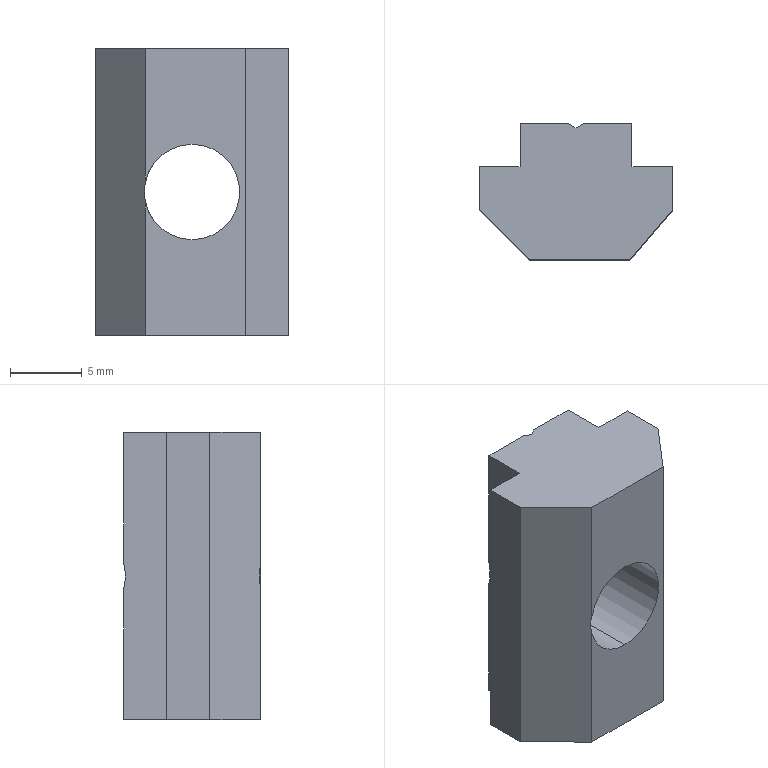Part | SolidWorks | features BaseBody 1 | 1 solid | 23 faces | box 13.5 x 9.5 x 20 mm | volume 1659 mm3 | plane 19 | cylinder 2 | cone 2 | commonest cylinder face diameters 6.647 x2
STEP:
#1=CARTESIAN_POINT('',(0.,0.,-3.324));
#2=VERTEX_POINT('',#1);
#3=CARTESIAN_POINT('',(-3.25,0.,-0.6951));
#4=VERTEX_POINT('',#3);
#5=CARTESIAN_POINT('',(0.,0.,0.));
#6=DIRECTION('',(0.,1.,0.));
#7=DIRECTION('',(0.,0.,1.));
#8=AXIS2_PLACEMENT_3D('',#5,#6,#7);
#9=CIRCLE('',#8,3.324);
#10=EDGE_CURVE('',#2,#4,#9,.T.);
#11=ORIENTED_EDGE('',*,*,#10,.F.);
#12=CARTESIAN_POINT('',(0.,8.823,-3.324));
#13=VERTEX_POINT('',#12);
#14=CARTESIAN_POINT('',(0.,0.,-3.324));
#15=DIRECTION('',(0.,1.,0.));
#16=VECTOR('',#15,1000.);
#17=LINE('',#14,#16);
#18=EDGE_CURVE('',#2,#13,#17,.T.);
#19=ORIENTED_EDGE('',*,*,#18,.T.);
#20=CARTESIAN_POINT('',(0.,8.823,3.324));
#21=VERTEX_POINT('',#20);
#22=CARTESIAN_POINT('',(0.,8.823,0.));
#23=DIRECTION('',(0.,-1.,0.));
#24=DIRECTION('',(0.,0.,1.));
#25=AXIS2_PLACEMENT_3D('',#22,#23,#24);
#26=CIRCLE('',#25,3.324);
#27=EDGE_CURVE('',#21,#13,#26,.T.);
#28=ORIENTED_EDGE('',*,*,#27,.F.);
#29=CARTESIAN_POINT('',(0.,0.,3.324));
#30=VERTEX_POINT('',#29);
#31=CARTESIAN_POINT('',(0.,0.,3.324));
#32=DIRECTION('',(0.,1.,0.));
#33=VECTOR('',#32,1000.);
#34=LINE('',#31,#33);
#35=EDGE_CURVE('',#30,#21,#34,.T.);
#36=ORIENTED_EDGE('',*,*,#35,.F.);
#37=CARTESIAN_POINT('',(-3.25,0.,0.6951));
#38=VERTEX_POINT('',#37);
#39=CARTESIAN_POINT('',(0.,0.,0.));
#40=DIRECTION('',(0.,1.,0.));
#41=DIRECTION('',(0.,0.,1.));
#42=AXIS2_PLACEMENT_3D('',#39,#40,#41);
#43=CIRCLE('',#42,3.324);
#44=EDGE_CURVE('',#38,#30,#43,.T.);
#45=ORIENTED_EDGE('',*,*,#44,.F.);
#46=CARTESIAN_POINT('',(-3.25,0.,0.6951));
#47=CARTESIAN_POINT('',(-3.348,0.09837,0.2352));
#48=CARTESIAN_POINT('',(-3.348,0.09837,-0.2352));
#49=CARTESIAN_POINT('',(-3.25,0.,-0.6951));
#50=(BOUNDED_CURVE()B_SPLINE_CURVE(3,(#46,#47,#48,#49),.UNSPECIFIED.,.F.,.F.)B_SPLINE_CURVE_WITH_KNOTS((4,4),(6.072,6.494),.UNSPECIFIED.)CURVE()GEOMETRIC_REPRESENTATION_ITEM()RATIONAL_B_SPLINE_CURVE((1.,0.9853,0.9853,1.))REPRESENTATION_ITEM(''));
#51=EDGE_CURVE('',#38,#4,#50,.T.);
#52=ORIENTED_EDGE('',*,*,#51,.T.);
#53=EDGE_LOOP('',(#11,#19,#28,#36,#45,#52));
#54=FACE_OUTER_BOUND('',#53,.T.);
#55=CARTESIAN_POINT('',(0.,0.,0.));
#56=DIRECTION('',(0.,1.,0.));
#57=DIRECTION('',(0.,0.,1.));
#58=AXIS2_PLACEMENT_3D('',#55,#56,#57);
#59=CYLINDRICAL_SURFACE('',#58,3.324);
#60=ADVANCED_FACE('',(#54),#59,.F.);
#61=ORIENTED_EDGE('',*,*,#27,.T.);
#62=CARTESIAN_POINT('',(0.,9.2,-3.7));
#63=VERTEX_POINT('',#62);
#64=CARTESIAN_POINT('',(0.,9.5,-4.));
#65=DIRECTION('',(0.,0.7071,-0.7071));
#66=VECTOR('',#65,1000.);
#67=LINE('',#64,#66);
#68=EDGE_CURVE('',#13,#63,#67,.T.);
#69=ORIENTED_EDGE('',*,*,#68,.T.);
#70=CARTESIAN_POINT('',(-0.5,9.5,-3.969));
#71=VERTEX_POINT('',#70);
#72=CARTESIAN_POINT('',(0.,9.2,-3.7));
#73=CARTESIAN_POINT('',(-0.1608,9.296,-3.796));
#74=CARTESIAN_POINT('',(-0.3276,9.397,-3.886));
#75=CARTESIAN_POINT('',(-0.5,9.5,-3.969));
#76=(BOUNDED_CURVE()B_SPLINE_CURVE(3,(#72,#73,#74,#75),.UNSPECIFIED.,.F.,.F.)B_SPLINE_CURVE_WITH_KNOTS((4,4),(4.069,4.173),.UNSPECIFIED.)CURVE()GEOMETRIC_REPRESENTATION_ITEM()RATIONAL_B_SPLINE_CURVE((1.,0.9991,0.9991,1.))REPRESENTATION_ITEM(''));
#77=EDGE_CURVE('',#63,#71,#76,.T.);
#78=ORIENTED_EDGE('',*,*,#77,.T.);
#79=CARTESIAN_POINT('',(-3.9,9.5,-0.8888));
#80=VERTEX_POINT('',#79);
#81=CARTESIAN_POINT('',(0.,9.5,0.));
#82=DIRECTION('',(0.,-1.,0.));
#83=DIRECTION('',(0.,0.,1.));
#84=AXIS2_PLACEMENT_3D('',#81,#82,#83);
#85=CIRCLE('',#84,4.);
#86=EDGE_CURVE('',#80,#71,#85,.T.);
#87=ORIENTED_EDGE('',*,*,#86,.F.);
#88=CARTESIAN_POINT('',(-3.9,9.5,0.8888));
#89=VERTEX_POINT('',#88);
#90=CARTESIAN_POINT('',(-3.9,9.5,0.8888));
#91=CARTESIAN_POINT('',(-3.9,9.435,0.5958));
#92=CARTESIAN_POINT('',(-3.9,9.4,0.3005));
#93=CARTESIAN_POINT('',(-3.9,9.4,-0.2953));
#94=CARTESIAN_POINT('',(-3.9,9.435,-0.5956));
#95=CARTESIAN_POINT('',(-3.9,9.5,-0.8888));
#96=B_SPLINE_CURVE_WITH_KNOTS('',3,(#90,#91,#92,#93,#94,#95),.UNSPECIFIED.,.F.,.F.,(4,2,4),(0.,0.0008912,0.001782),.UNSPECIFIED.);
#97=EDGE_CURVE('',#89,#80,#96,.T.);
#98=ORIENTED_EDGE('',*,*,#97,.F.);
#99=CARTESIAN_POINT('',(-0.5,9.5,3.969));
#100=VERTEX_POINT('',#99);
#101=CARTESIAN_POINT('',(0.,9.5,0.));
#102=DIRECTION('',(0.,-1.,0.));
#103=DIRECTION('',(0.,0.,1.));
#104=AXIS2_PLACEMENT_3D('',#101,#102,#103);
#105=CIRCLE('',#104,4.);
#106=EDGE_CURVE('',#100,#89,#105,.T.);
#107=ORIENTED_EDGE('',*,*,#106,.F.);
#108=CARTESIAN_POINT('',(0.,9.2,3.7));
#109=VERTEX_POINT('',#108);
#110=CARTESIAN_POINT('',(-0.5,9.5,3.969));
#111=CARTESIAN_POINT('',(-0.3276,9.397,3.886));
#112=CARTESIAN_POINT('',(-0.1608,9.296,3.796));
#113=CARTESIAN_POINT('',(0.,9.2,3.7));
#114=(BOUNDED_CURVE()B_SPLINE_CURVE(3,(#110,#111,#112,#113),.UNSPECIFIED.,.F.,.F.)B_SPLINE_CURVE_WITH_KNOTS((4,4),(2.11,2.214),.UNSPECIFIED.)CURVE()GEOMETRIC_REPRESENTATION_ITEM()RATIONAL_B_SPLINE_CURVE((1.,0.9991,0.9991,1.))REPRESENTATION_ITEM(''));
#115=EDGE_CURVE('',#100,#109,#114,.T.);
#116=ORIENTED_EDGE('',*,*,#115,.T.);
#117=CARTESIAN_POINT('',(0.,9.5,4.));
#118=DIRECTION('',(0.,0.7071,0.7071));
#119=VECTOR('',#118,1000.);
#120=LINE('',#117,#119);
#121=EDGE_CURVE('',#21,#109,#120,.T.);
#122=ORIENTED_EDGE('',*,*,#121,.F.);
#123=EDGE_LOOP('',(#61,#69,#78,#87,#98,#107,#116,#122));
#124=FACE_OUTER_BOUND('',#123,.T.);
#125=CARTESIAN_POINT('',(0.,9.5,0.));
#126=DIRECTION('',(0.,1.,0.));
#127=DIRECTION('',(0.,0.,1.));
#128=AXIS2_PLACEMENT_3D('',#125,#126,#127);
#129=CONICAL_SURFACE('',#128,4.,0.7854);
#130=ADVANCED_FACE('',(#124),#129,.F.);
#131=ORIENTED_EDGE('',*,*,#18,.F.);
#132=CARTESIAN_POINT('',(0.,0.,0.));
#133=DIRECTION('',(0.,1.,0.));
#134=DIRECTION('',(0.,0.,1.));
#135=AXIS2_PLACEMENT_3D('',#132,#133,#134);
#136=CIRCLE('',#135,3.324);
#137=EDGE_CURVE('',#30,#2,#136,.T.);
#138=ORIENTED_EDGE('',*,*,#137,.F.);
#139=ORIENTED_EDGE('',*,*,#35,.T.);
#140=CARTESIAN_POINT('',(0.,8.823,0.));
#141=DIRECTION('',(0.,-1.,0.));
#142=DIRECTION('',(0.,0.,1.));
#143=AXIS2_PLACEMENT_3D('',#140,#141,#142);
#144=CIRCLE('',#143,3.324);
#145=EDGE_CURVE('',#13,#21,#144,.T.);
#146=ORIENTED_EDGE('',*,*,#145,.F.);
#147=EDGE_LOOP('',(#131,#138,#139,#146));
#148=FACE_OUTER_BOUND('',#147,.T.);
#149=CARTESIAN_POINT('',(0.,0.,0.));
#150=DIRECTION('',(0.,1.,0.));
#151=DIRECTION('',(0.,0.,1.));
#152=AXIS2_PLACEMENT_3D('',#149,#150,#151);
#153=CYLINDRICAL_SURFACE('',#152,3.324);
#154=ADVANCED_FACE('',(#148),#153,.F.);
#155=ORIENTED_EDGE('',*,*,#68,.F.);
#156=ORIENTED_EDGE('',*,*,#145,.T.);
#157=ORIENTED_EDGE('',*,*,#121,.T.);
#158=CARTESIAN_POINT('',(0.5,9.5,3.969));
#159=VERTEX_POINT('',#158);
#160=CARTESIAN_POINT('',(0.,9.2,3.7));
#161=CARTESIAN_POINT('',(0.1608,9.296,3.796));
#162=CARTESIAN_POINT('',(0.3276,9.397,3.886));
#163=CARTESIAN_POINT('',(0.5,9.5,3.969));
#164=(BOUNDED_CURVE()B_SPLINE_CURVE(3,(#160,#161,#162,#163),.UNSPECIFIED.,.F.,.F.)B_SPLINE_CURVE_WITH_KNOTS((4,4),(4.069,4.173),.UNSPECIFIED.)CURVE()GEOMETRIC_REPRESENTATION_ITEM()RATIONAL_B_SPLINE_CURVE((1.,0.9991,0.9991,1.))REPRESENTATION_ITEM(''));
#165=EDGE_CURVE('',#109,#159,#164,.T.);
#166=ORIENTED_EDGE('',*,*,#165,.T.);
#167=CARTESIAN_POINT('',(3.9,9.5,0.8888));
#168=VERTEX_POINT('',#167);
#169=CARTESIAN_POINT('',(0.,9.5,0.));
#170=DIRECTION('',(0.,-1.,0.));
#171=DIRECTION('',(0.,0.,1.));
#172=AXIS2_PLACEMENT_3D('',#169,#170,#171);
#173=CIRCLE('',#172,4.);
#174=EDGE_CURVE('',#168,#159,#173,.T.);
#175=ORIENTED_EDGE('',*,*,#174,.F.);
#176=CARTESIAN_POINT('',(3.9,9.5,-0.8888));
#177=VERTEX_POINT('',#176);
#178=CARTESIAN_POINT('',(3.9,9.5,-0.8888));
#179=CARTESIAN_POINT('',(3.9,9.435,-0.5958));
#180=CARTESIAN_POINT('',(3.9,9.4,-0.3005));
#181=CARTESIAN_POINT('',(3.9,9.4,0.2953));
#182=CARTESIAN_POINT('',(3.9,9.435,0.5956));
#183=CARTESIAN_POINT('',(3.9,9.5,0.8888));
#184=B_SPLINE_CURVE_WITH_KNOTS('',3,(#178,#179,#180,#181,#182,#183),.UNSPECIFIED.,.F.,.F.,(4,2,4),(0.,0.0008912,0.001782),.UNSPECIFIED.);
#185=EDGE_CURVE('',#177,#168,#184,.T.);
#186=ORIENTED_EDGE('',*,*,#185,.F.);
#187=CARTESIAN_POINT('',(0.5,9.5,-3.969));
#188=VERTEX_POINT('',#187);
#189=CARTESIAN_POINT('',(0.,9.5,0.));
#190=DIRECTION('',(0.,-1.,0.));
#191=DIRECTION('',(0.,0.,1.));
#192=AXIS2_PLACEMENT_3D('',#189,#190,#191);
#193=CIRCLE('',#192,4.);
#194=EDGE_CURVE('',#188,#177,#193,.T.);
#195=ORIENTED_EDGE('',*,*,#194,.F.);
#196=CARTESIAN_POINT('',(0.5,9.5,-3.969));
#197=CARTESIAN_POINT('',(0.3276,9.397,-3.886));
#198=CARTESIAN_POINT('',(0.1608,9.296,-3.796));
#199=CARTESIAN_POINT('',(0.,9.2,-3.7));
#200=(BOUNDED_CURVE()B_SPLINE_CURVE(3,(#196,#197,#198,#199),.UNSPECIFIED.,.F.,.F.)B_SPLINE_CURVE_WITH_KNOTS((4,4),(2.11,2.214),.UNSPECIFIED.)CURVE()GEOMETRIC_REPRESENTATION_ITEM()RATIONAL_B_SPLINE_CURVE((1.,0.9991,0.9991,1.))REPRESENTATION_ITEM(''));
#201=EDGE_CURVE('',#188,#63,#200,.T.);
#202=ORIENTED_EDGE('',*,*,#201,.T.);
#203=EDGE_LOOP('',(#155,#156,#157,#166,#175,#186,#195,#202));
#204=FACE_OUTER_BOUND('',#203,.T.);
#205=CARTESIAN_POINT('',(0.,9.5,0.));
#206=DIRECTION('',(0.,1.,0.));
#207=DIRECTION('',(0.,0.,1.));
#208=AXIS2_PLACEMENT_3D('',#205,#206,#207);
#209=CONICAL_SURFACE('',#208,4.,0.7854);
#210=ADVANCED_FACE('',(#204),#209,.F.);
#211=ORIENTED_EDGE('',*,*,#44,.T.);
#212=ORIENTED_EDGE('',*,*,#137,.T.);
#213=ORIENTED_EDGE('',*,*,#10,.T.);
#214=CARTESIAN_POINT('',(-3.25,0.,-10.));
#215=VERTEX_POINT('',#214);
#216=CARTESIAN_POINT('',(-3.25,0.,10.));
#217=DIRECTION('',(0.,0.,1.));
#218=VECTOR('',#217,1000.);
#219=LINE('',#216,#218);
#220=EDGE_CURVE('',#215,#4,#219,.T.);
#221=ORIENTED_EDGE('',*,*,#220,.F.);
#222=CARTESIAN_POINT('',(3.75,0.,-10.));
#223=VERTEX_POINT('',#222);
#224=CARTESIAN_POINT('',(-3.25,0.,-10.));
#225=DIRECTION('',(-1.,0.,0.));
#226=VECTOR('',#225,1000.);
#227=LINE('',#224,#226);
#228=EDGE_CURVE('',#223,#215,#227,.T.);
#229=ORIENTED_EDGE('',*,*,#228,.F.);
#230=CARTESIAN_POINT('',(3.75,0.,10.));
#231=VERTEX_POINT('',#230);
#232=CARTESIAN_POINT('',(3.75,0.,10.));
#233=DIRECTION('',(0.,0.,-1.));
#234=VECTOR('',#233,1000.);
#235=LINE('',#232,#234);
#236=EDGE_CURVE('',#231,#223,#235,.T.);
#237=ORIENTED_EDGE('',*,*,#236,.F.);
#238=CARTESIAN_POINT('',(-3.25,0.,10.));
#239=VERTEX_POINT('',#238);
#240=CARTESIAN_POINT('',(-3.25,0.,10.));
#241=DIRECTION('',(1.,0.,0.));
#242=VECTOR('',#241,1000.);
#243=LINE('',#240,#242);
#244=EDGE_CURVE('',#239,#231,#243,.T.);
#245=ORIENTED_EDGE('',*,*,#244,.F.);
#246=CARTESIAN_POINT('',(-3.25,0.,10.));
#247=DIRECTION('',(0.,0.,1.));
#248=VECTOR('',#247,1000.);
#249=LINE('',#246,#248);
#250=EDGE_CURVE('',#38,#239,#249,.T.);
#251=ORIENTED_EDGE('',*,*,#250,.F.);
#252=EDGE_LOOP('',(#211,#212,#213,#221,#229,#237,#245,#251));
#253=FACE_OUTER_BOUND('',#252,.T.);
#254=CARTESIAN_POINT('',(-3.25,0.,10.));
#255=DIRECTION('',(0.,1.,0.));
#256=DIRECTION('',(0.,0.,1.));
#257=AXIS2_PLACEMENT_3D('',#254,#255,#256);
#258=PLANE('',#257);
#259=ADVANCED_FACE('',(#253),#258,.F.);
#260=CARTESIAN_POINT('',(3.9,9.5,10.));
#261=VERTEX_POINT('',#260);
#262=CARTESIAN_POINT('',(3.9,9.5,10.));
#263=DIRECTION('',(0.,0.,-1.));
#264=VECTOR('',#263,1000.);
#265=LINE('',#262,#264);
#266=EDGE_CURVE('',#261,#168,#265,.T.);
#267=ORIENTED_EDGE('',*,*,#266,.F.);
#268=CARTESIAN_POINT('',(3.9,6.5,10.));
#269=VERTEX_POINT('',#268);
#270=CARTESIAN_POINT('',(3.9,6.5,10.));
#271=DIRECTION('',(0.,1.,0.));
#272=VECTOR('',#271,1000.);
#273=LINE('',#270,#272);
#274=EDGE_CURVE('',#269,#261,#273,.T.);
#275=ORIENTED_EDGE('',*,*,#274,.F.);
#276=CARTESIAN_POINT('',(3.9,6.5,-10.));
#277=VERTEX_POINT('',#276);
#278=CARTESIAN_POINT('',(3.9,6.5,10.));
#279=DIRECTION('',(0.,0.,1.));
#280=VECTOR('',#279,1000.);
#281=LINE('',#278,#280);
#282=EDGE_CURVE('',#277,#269,#281,.T.);
#283=ORIENTED_EDGE('',*,*,#282,.F.);
#284=CARTESIAN_POINT('',(3.9,9.5,-10.));
#285=VERTEX_POINT('',#284);
#286=CARTESIAN_POINT('',(3.9,6.5,-10.));
#287=DIRECTION('',(0.,-1.,0.));
#288=VECTOR('',#287,1000.);
#289=LINE('',#286,#288);
#290=EDGE_CURVE('',#285,#277,#289,.T.);
#291=ORIENTED_EDGE('',*,*,#290,.F.);
#292=CARTESIAN_POINT('',(3.9,9.5,10.));
#293=DIRECTION('',(0.,0.,-1.));
#294=VECTOR('',#293,1000.);
#295=LINE('',#292,#294);
#296=EDGE_CURVE('',#177,#285,#295,.T.);
#297=ORIENTED_EDGE('',*,*,#296,.F.);
#298=ORIENTED_EDGE('',*,*,#185,.T.);
#299=EDGE_LOOP('',(#267,#275,#283,#291,#297,#298));
#300=FACE_OUTER_BOUND('',#299,.T.);
#301=CARTESIAN_POINT('',(3.9,6.5,10.));
#302=DIRECTION('',(-1.,0.,0.));
#303=DIRECTION('',(0.,-1.,0.));
#304=AXIS2_PLACEMENT_3D('',#301,#302,#303);
#305=PLANE('',#304);
#306=ADVANCED_FACE('',(#300),#305,.F.);
#307=ORIENTED_EDGE('',*,*,#296,.T.);
#308=CARTESIAN_POINT('',(0.5,9.5,-10.));
#309=VERTEX_POINT('',#308);
#310=CARTESIAN_POINT('',(3.9,9.5,-10.));
#311=DIRECTION('',(1.,0.,0.));
#312=VECTOR('',#311,1000.);
#313=LINE('',#310,#312);
#314=EDGE_CURVE('',#309,#285,#313,.T.);
#315=ORIENTED_EDGE('',*,*,#314,.F.);
#316=CARTESIAN_POINT('',(0.5,9.5,10.));
#317=DIRECTION('',(0.,0.,-1.));
#318=VECTOR('',#317,1000.);
#319=LINE('',#316,#318);
#320=EDGE_CURVE('',#188,#309,#319,.T.);
#321=ORIENTED_EDGE('',*,*,#320,.F.);
#322=ORIENTED_EDGE('',*,*,#194,.T.);
#323=EDGE_LOOP('',(#307,#315,#321,#322));
#324=FACE_OUTER_BOUND('',#323,.T.);
#325=CARTESIAN_POINT('',(3.9,9.5,10.));
#326=DIRECTION('',(0.,-1.,0.));
#327=DIRECTION('',(0.,0.,-1.));
#328=AXIS2_PLACEMENT_3D('',#325,#326,#327);
#329=PLANE('',#328);
#330=ADVANCED_FACE('',(#324),#329,.F.);
#331=CARTESIAN_POINT('',(-0.5,9.5,-10.));
#332=VERTEX_POINT('',#331);
#333=CARTESIAN_POINT('',(-0.5,9.5,10.));
#334=DIRECTION('',(0.,0.,1.));
#335=VECTOR('',#334,1000.);
#336=LINE('',#333,#335);
#337=EDGE_CURVE('',#332,#71,#336,.T.);
#338=ORIENTED_EDGE('',*,*,#337,.F.);
#339=CARTESIAN_POINT('',(-3.9,9.5,-10.));
#340=VERTEX_POINT('',#339);
#341=CARTESIAN_POINT('',(-0.5,9.5,-10.));
#342=DIRECTION('',(1.,0.,0.));
#343=VECTOR('',#342,1000.);
#344=LINE('',#341,#343);
#345=EDGE_CURVE('',#340,#332,#344,.T.);
#346=ORIENTED_EDGE('',*,*,#345,.F.);
#347=CARTESIAN_POINT('',(-3.9,9.5,10.));
#348=DIRECTION('',(0.,0.,-1.));
#349=VECTOR('',#348,1000.);
#350=LINE('',#347,#349);
#351=EDGE_CURVE('',#80,#340,#350,.T.);
#352=ORIENTED_EDGE('',*,*,#351,.F.);
#353=ORIENTED_EDGE('',*,*,#86,.T.);
#354=EDGE_LOOP('',(#338,#346,#352,#353));
#355=FACE_OUTER_BOUND('',#354,.T.);
#356=CARTESIAN_POINT('',(-0.5,9.5,10.));
#357=DIRECTION('',(0.,-1.,0.));
#358=DIRECTION('',(0.,0.,-1.));
#359=AXIS2_PLACEMENT_3D('',#356,#357,#358);
#360=PLANE('',#359);
#361=ADVANCED_FACE('',(#355),#360,.F.);
#362=ORIENTED_EDGE('',*,*,#351,.T.);
#363=CARTESIAN_POINT('',(-3.9,6.5,-10.));
#364=VERTEX_POINT('',#363);
#365=CARTESIAN_POINT('',(-3.9,9.5,-10.));
#366=DIRECTION('',(0.,1.,0.));
#367=VECTOR('',#366,1000.);
#368=LINE('',#365,#367);
#369=EDGE_CURVE('',#364,#340,#368,.T.);
#370=ORIENTED_EDGE('',*,*,#369,.F.);
#371=CARTESIAN_POINT('',(-3.9,6.5,10.));
#372=VERTEX_POINT('',#371);
#373=CARTESIAN_POINT('',(-3.9,6.5,10.));
#374=DIRECTION('',(0.,0.,-1.));
#375=VECTOR('',#374,1000.);
#376=LINE('',#373,#375);
#377=EDGE_CURVE('',#372,#364,#376,.T.);
#378=ORIENTED_EDGE('',*,*,#377,.F.);
#379=CARTESIAN_POINT('',(-3.9,9.5,10.));
#380=VERTEX_POINT('',#379);
#381=CARTESIAN_POINT('',(-3.9,9.5,10.));
#382=DIRECTION('',(0.,-1.,0.));
#383=VECTOR('',#382,1000.);
#384=LINE('',#381,#383);
#385=EDGE_CURVE('',#380,#372,#384,.T.);
#386=ORIENTED_EDGE('',*,*,#385,.F.);
#387=CARTESIAN_POINT('',(-3.9,9.5,10.));
#388=DIRECTION('',(0.,0.,1.));
#389=VECTOR('',#388,1000.);
#390=LINE('',#387,#389);
#391=EDGE_CURVE('',#89,#380,#390,.T.);
#392=ORIENTED_EDGE('',*,*,#391,.F.);
#393=ORIENTED_EDGE('',*,*,#97,.T.);
#394=EDGE_LOOP('',(#362,#370,#378,#386,#392,#393));
#395=FACE_OUTER_BOUND('',#394,.T.);
#396=CARTESIAN_POINT('',(-3.9,9.5,10.));
#397=DIRECTION('',(1.,0.,0.));
#398=DIRECTION('',(0.,1.,0.));
#399=AXIS2_PLACEMENT_3D('',#396,#397,#398);
#400=PLANE('',#399);
#401=ADVANCED_FACE('',(#395),#400,.F.);
#402=ORIENTED_EDGE('',*,*,#391,.T.);
#403=CARTESIAN_POINT('',(-0.5,9.5,10.));
#404=VERTEX_POINT('',#403);
#405=CARTESIAN_POINT('',(-0.5,9.5,10.));
#406=DIRECTION('',(-1.,0.,0.));
#407=VECTOR('',#406,1000.);
#408=LINE('',#405,#407);
#409=EDGE_CURVE('',#404,#380,#408,.T.);
#410=ORIENTED_EDGE('',*,*,#409,.F.);
#411=CARTESIAN_POINT('',(-0.5,9.5,10.));
#412=DIRECTION('',(0.,0.,1.));
#413=VECTOR('',#412,1000.);
#414=LINE('',#411,#413);
#415=EDGE_CURVE('',#100,#404,#414,.T.);
#416=ORIENTED_EDGE('',*,*,#415,.F.);
#417=ORIENTED_EDGE('',*,*,#106,.T.);
#418=EDGE_LOOP('',(#402,#410,#416,#417));
#419=FACE_OUTER_BOUND('',#418,.T.);
#420=CARTESIAN_POINT('',(-0.5,9.5,10.));
#421=DIRECTION('',(0.,-1.,0.));
#422=DIRECTION('',(0.,0.,-1.));
#423=AXIS2_PLACEMENT_3D('',#420,#421,#422);
#424=PLANE('',#423);
#425=ADVANCED_FACE('',(#419),#424,.F.);
#426=CARTESIAN_POINT('',(0.5,9.5,10.));
#427=VERTEX_POINT('',#426);
#428=CARTESIAN_POINT('',(0.5,9.5,10.));
#429=DIRECTION('',(0.,0.,-1.));
#430=VECTOR('',#429,1000.);
#431=LINE('',#428,#430);
#432=EDGE_CURVE('',#427,#159,#431,.T.);
#433=ORIENTED_EDGE('',*,*,#432,.F.);
#434=CARTESIAN_POINT('',(3.9,9.5,10.));
#435=DIRECTION('',(-1.,0.,0.));
#436=VECTOR('',#435,1000.);
#437=LINE('',#434,#436);
#438=EDGE_CURVE('',#261,#427,#437,.T.);
#439=ORIENTED_EDGE('',*,*,#438,.F.);
#440=ORIENTED_EDGE('',*,*,#266,.T.);
#441=ORIENTED_EDGE('',*,*,#174,.T.);
#442=EDGE_LOOP('',(#433,#439,#440,#441));
#443=FACE_OUTER_BOUND('',#442,.T.);
#444=CARTESIAN_POINT('',(3.9,9.5,10.));
#445=DIRECTION('',(0.,-1.,0.));
#446=DIRECTION('',(0.,0.,-1.));
#447=AXIS2_PLACEMENT_3D('',#444,#445,#446);
#448=PLANE('',#447);
#449=ADVANCED_FACE('',(#443),#448,.F.);
#450=ORIENTED_EDGE('',*,*,#250,.T.);
#451=CARTESIAN_POINT('',(-6.75,3.5,10.));
#452=VERTEX_POINT('',#451);
#453=CARTESIAN_POINT('',(-6.75,3.5,10.));
#454=DIRECTION('',(0.7071,-0.7071,0.));
#455=VECTOR('',#454,1000.);
#456=LINE('',#453,#455);
#457=EDGE_CURVE('',#452,#239,#456,.T.);
#458=ORIENTED_EDGE('',*,*,#457,.F.);
#459=CARTESIAN_POINT('',(-6.75,3.5,-10.));
#460=VERTEX_POINT('',#459);
#461=CARTESIAN_POINT('',(-6.75,3.5,10.));
#462=DIRECTION('',(0.,0.,1.));
#463=VECTOR('',#462,1000.);
#464=LINE('',#461,#463);
#465=EDGE_CURVE('',#460,#452,#464,.T.);
#466=ORIENTED_EDGE('',*,*,#465,.F.);
#467=CARTESIAN_POINT('',(-6.75,3.5,-10.));
#468=DIRECTION('',(-0.7071,0.7071,0.));
#469=VECTOR('',#468,1000.);
#470=LINE('',#467,#469);
#471=EDGE_CURVE('',#215,#460,#470,.T.);
#472=ORIENTED_EDGE('',*,*,#471,.F.);
#473=ORIENTED_EDGE('',*,*,#220,.T.);
#474=ORIENTED_EDGE('',*,*,#51,.F.);
#475=EDGE_LOOP('',(#450,#458,#466,#472,#473,#474));
#476=FACE_OUTER_BOUND('',#475,.T.);
#477=CARTESIAN_POINT('',(-6.75,3.5,10.));
#478=DIRECTION('',(0.7071,0.7071,0.));
#479=DIRECTION('',(-0.7071,0.7071,0.));
#480=AXIS2_PLACEMENT_3D('',#477,#478,#479);
#481=PLANE('',#480);
#482=ADVANCED_FACE('',(#476),#481,.F.);
#483=CARTESIAN_POINT('',(-6.75,6.5,-10.));
#484=VERTEX_POINT('',#483);
#485=CARTESIAN_POINT('',(0.,6.5,-10.));
#486=DIRECTION('',(-1.,0.,0.));
#487=VECTOR('',#486,1000.);
#488=LINE('',#485,#487);
#489=EDGE_CURVE('',#364,#484,#488,.T.);
#490=ORIENTED_EDGE('',*,*,#489,.F.);
#491=ORIENTED_EDGE('',*,*,#369,.T.);
#492=ORIENTED_EDGE('',*,*,#345,.T.);
#493=CARTESIAN_POINT('',(0.,9.2,-10.));
#494=VERTEX_POINT('',#493);
#495=CARTESIAN_POINT('',(0.,9.2,-10.));
#496=DIRECTION('',(-0.8575,0.5145,0.));
#497=VECTOR('',#496,1000.);
#498=LINE('',#495,#497);
#499=EDGE_CURVE('',#494,#332,#498,.T.);
#500=ORIENTED_EDGE('',*,*,#499,.F.);
#501=CARTESIAN_POINT('',(0.5,9.5,-10.));
#502=DIRECTION('',(-0.8575,-0.5145,0.));
#503=VECTOR('',#502,1000.);
#504=LINE('',#501,#503);
#505=EDGE_CURVE('',#309,#494,#504,.T.);
#506=ORIENTED_EDGE('',*,*,#505,.F.);
#507=ORIENTED_EDGE('',*,*,#314,.T.);
#508=ORIENTED_EDGE('',*,*,#290,.T.);
#509=CARTESIAN_POINT('',(6.75,6.5,-10.));
#510=VERTEX_POINT('',#509);
#511=CARTESIAN_POINT('',(0.,6.5,-10.));
#512=DIRECTION('',(-1.,0.,0.));
#513=VECTOR('',#512,1000.);
#514=LINE('',#511,#513);
#515=EDGE_CURVE('',#510,#277,#514,.T.);
#516=ORIENTED_EDGE('',*,*,#515,.F.);
#517=CARTESIAN_POINT('',(6.75,3.5,-10.));
#518=VERTEX_POINT('',#517);
#519=CARTESIAN_POINT('',(6.75,0.,-10.));
#520=DIRECTION('',(0.,1.,0.));
#521=VECTOR('',#520,1000.);
#522=LINE('',#519,#521);
#523=EDGE_CURVE('',#518,#510,#522,.T.);
#524=ORIENTED_EDGE('',*,*,#523,.F.);
#525=CARTESIAN_POINT('',(3.75,0.,-10.));
#526=DIRECTION('',(0.6508,0.7593,0.));
#527=VECTOR('',#526,1000.);
#528=LINE('',#525,#527);
#529=EDGE_CURVE('',#223,#518,#528,.T.);
#530=ORIENTED_EDGE('',*,*,#529,.F.);
#531=ORIENTED_EDGE('',*,*,#228,.T.);
#532=ORIENTED_EDGE('',*,*,#471,.T.);
#533=CARTESIAN_POINT('',(-6.75,0.,-10.));
#534=DIRECTION('',(0.,-1.,0.));
#535=VECTOR('',#534,1000.);
#536=LINE('',#533,#535);
#537=EDGE_CURVE('',#484,#460,#536,.T.);
#538=ORIENTED_EDGE('',*,*,#537,.F.);
#539=EDGE_LOOP('',(#490,#491,#492,#500,#506,#507,#508,#516,#524,#530,#531,#532,#538));
#540=FACE_OUTER_BOUND('',#539,.T.);
#541=CARTESIAN_POINT('',(0.,0.,-10.));
#542=DIRECTION('',(0.,0.,1.));
#543=DIRECTION('',(1.,0.,0.));
#544=AXIS2_PLACEMENT_3D('',#541,#542,#543);
#545=PLANE('',#544);
#546=ADVANCED_FACE('',(#540),#545,.F.);
#547=CARTESIAN_POINT('',(6.75,3.5,10.));
#548=VERTEX_POINT('',#547);
#549=CARTESIAN_POINT('',(6.75,3.5,10.));
#550=DIRECTION('',(0.,0.,-1.));
#551=VECTOR('',#550,1000.);
#552=LINE('',#549,#551);
#553=EDGE_CURVE('',#548,#518,#552,.T.);
#554=ORIENTED_EDGE('',*,*,#553,.F.);
#555=CARTESIAN_POINT('',(3.75,0.,10.));
#556=DIRECTION('',(0.6508,0.7593,0.));
#557=VECTOR('',#556,1000.);
#558=LINE('',#555,#557);
#559=EDGE_CURVE('',#231,#548,#558,.T.);
#560=ORIENTED_EDGE('',*,*,#559,.F.);
#561=ORIENTED_EDGE('',*,*,#236,.T.);
#562=ORIENTED_EDGE('',*,*,#529,.T.);
#563=EDGE_LOOP('',(#554,#560,#561,#562));
#564=FACE_OUTER_BOUND('',#563,.T.);
#565=CARTESIAN_POINT('',(3.75,0.,10.));
#566=DIRECTION('',(-0.7593,0.6508,0.));
#567=DIRECTION('',(-0.6508,-0.7593,0.));
#568=AXIS2_PLACEMENT_3D('',#565,#566,#567);
#569=PLANE('',#568);
#570=ADVANCED_FACE('',(#564),#569,.F.);
#571=ORIENTED_EDGE('',*,*,#385,.T.);
#572=CARTESIAN_POINT('',(-6.75,6.5,10.));
#573=VERTEX_POINT('',#572);
#574=CARTESIAN_POINT('',(0.,6.5,10.));
#575=DIRECTION('',(-1.,0.,0.));
#576=VECTOR('',#575,1000.);
#577=LINE('',#574,#576);
#578=EDGE_CURVE('',#372,#573,#577,.T.);
#579=ORIENTED_EDGE('',*,*,#578,.T.);
#580=CARTESIAN_POINT('',(-6.75,0.,10.));
#581=DIRECTION('',(0.,-1.,0.));
#582=VECTOR('',#581,1000.);
#583=LINE('',#580,#582);
#584=EDGE_CURVE('',#573,#452,#583,.T.);
#585=ORIENTED_EDGE('',*,*,#584,.T.);
#586=ORIENTED_EDGE('',*,*,#457,.T.);
#587=ORIENTED_EDGE('',*,*,#244,.T.);
#588=ORIENTED_EDGE('',*,*,#559,.T.);
#589=CARTESIAN_POINT('',(6.75,6.5,10.));
#590=VERTEX_POINT('',#589);
#591=CARTESIAN_POINT('',(6.75,0.,10.));
#592=DIRECTION('',(0.,1.,0.));
#593=VECTOR('',#592,1000.);
#594=LINE('',#591,#593);
#595=EDGE_CURVE('',#548,#590,#594,.T.);
#596=ORIENTED_EDGE('',*,*,#595,.T.);
#597=CARTESIAN_POINT('',(0.,6.5,10.));
#598=DIRECTION('',(-1.,0.,0.));
#599=VECTOR('',#598,1000.);
#600=LINE('',#597,#599);
#601=EDGE_CURVE('',#590,#269,#600,.T.);
#602=ORIENTED_EDGE('',*,*,#601,.T.);
#603=ORIENTED_EDGE('',*,*,#274,.T.);
#604=ORIENTED_EDGE('',*,*,#438,.T.);
#605=CARTESIAN_POINT('',(0.,9.2,10.));
#606=VERTEX_POINT('',#605);
#607=CARTESIAN_POINT('',(0.5,9.5,10.));
#608=DIRECTION('',(-0.8575,-0.5145,0.));
#609=VECTOR('',#608,1000.);
#610=LINE('',#607,#609);
#611=EDGE_CURVE('',#427,#606,#610,.T.);
#612=ORIENTED_EDGE('',*,*,#611,.T.);
#613=CARTESIAN_POINT('',(0.,9.2,10.));
#614=DIRECTION('',(-0.8575,0.5145,0.));
#615=VECTOR('',#614,1000.);
#616=LINE('',#613,#615);
#617=EDGE_CURVE('',#606,#404,#616,.T.);
#618=ORIENTED_EDGE('',*,*,#617,.T.);
#619=ORIENTED_EDGE('',*,*,#409,.T.);
#620=EDGE_LOOP('',(#571,#579,#585,#586,#587,#588,#596,#602,#603,#604,#612,#618,#619));
#621=FACE_OUTER_BOUND('',#620,.T.);
#622=CARTESIAN_POINT('',(0.,0.,10.));
#623=DIRECTION('',(0.,0.,1.));
#624=DIRECTION('',(1.,0.,0.));
#625=AXIS2_PLACEMENT_3D('',#622,#623,#624);
#626=PLANE('',#625);
#627=ADVANCED_FACE('',(#621),#626,.T.);
#628=ORIENTED_EDGE('',*,*,#282,.T.);
#629=ORIENTED_EDGE('',*,*,#601,.F.);
#630=CARTESIAN_POINT('',(6.75,6.5,10.));
#631=DIRECTION('',(0.,0.,1.));
#632=VECTOR('',#631,1000.);
#633=LINE('',#630,#632);
#634=EDGE_CURVE('',#510,#590,#633,.T.);
#635=ORIENTED_EDGE('',*,*,#634,.F.);
#636=ORIENTED_EDGE('',*,*,#515,.T.);
#637=EDGE_LOOP('',(#628,#629,#635,#636));
#638=FACE_OUTER_BOUND('',#637,.T.);
#639=CARTESIAN_POINT('',(6.75,6.5,10.));
#640=DIRECTION('',(0.,-1.,0.));
#641=DIRECTION('',(0.,0.,-1.));
#642=AXIS2_PLACEMENT_3D('',#639,#640,#641);
#643=PLANE('',#642);
#644=ADVANCED_FACE('',(#638),#643,.F.);
#645=ORIENTED_EDGE('',*,*,#320,.T.);
#646=ORIENTED_EDGE('',*,*,#505,.T.);
#647=CARTESIAN_POINT('',(0.,9.2,10.));
#648=DIRECTION('',(0.,0.,-1.));
#649=VECTOR('',#648,1000.);
#650=LINE('',#647,#649);
#651=EDGE_CURVE('',#63,#494,#650,.T.);
#652=ORIENTED_EDGE('',*,*,#651,.F.);
#653=ORIENTED_EDGE('',*,*,#201,.F.);
#654=EDGE_LOOP('',(#645,#646,#652,#653));
#655=FACE_OUTER_BOUND('',#654,.T.);
#656=CARTESIAN_POINT('',(0.5,9.5,10.));
#657=DIRECTION('',(0.5145,-0.8575,0.));
#658=DIRECTION('',(0.8575,0.5145,0.));
#659=AXIS2_PLACEMENT_3D('',#656,#657,#658);
#660=PLANE('',#659);
#661=ADVANCED_FACE('',(#655),#660,.F.);
#662=ORIENTED_EDGE('',*,*,#651,.T.);
#663=ORIENTED_EDGE('',*,*,#499,.T.);
#664=ORIENTED_EDGE('',*,*,#337,.T.);
#665=ORIENTED_EDGE('',*,*,#77,.F.);
#666=EDGE_LOOP('',(#662,#663,#664,#665));
#667=FACE_OUTER_BOUND('',#666,.T.);
#668=CARTESIAN_POINT('',(0.,9.2,10.));
#669=DIRECTION('',(-0.5145,-0.8575,0.));
#670=DIRECTION('',(0.8575,-0.5145,0.));
#671=AXIS2_PLACEMENT_3D('',#668,#669,#670);
#672=PLANE('',#671);
#673=ADVANCED_FACE('',(#667),#672,.F.);
#674=CARTESIAN_POINT('',(-6.75,6.5,10.));
#675=DIRECTION('',(0.,0.,-1.));
#676=VECTOR('',#675,1000.);
#677=LINE('',#674,#676);
#678=EDGE_CURVE('',#573,#484,#677,.T.);
#679=ORIENTED_EDGE('',*,*,#678,.F.);
#680=ORIENTED_EDGE('',*,*,#578,.F.);
#681=ORIENTED_EDGE('',*,*,#377,.T.);
#682=ORIENTED_EDGE('',*,*,#489,.T.);
#683=EDGE_LOOP('',(#679,#680,#681,#682));
#684=FACE_OUTER_BOUND('',#683,.T.);
#685=CARTESIAN_POINT('',(-3.9,6.5,10.));
#686=DIRECTION('',(0.,-1.,0.));
#687=DIRECTION('',(0.,0.,-1.));
#688=AXIS2_PLACEMENT_3D('',#685,#686,#687);
#689=PLANE('',#688);
#690=ADVANCED_FACE('',(#684),#689,.F.);
#691=ORIENTED_EDGE('',*,*,#415,.T.);
#692=ORIENTED_EDGE('',*,*,#617,.F.);
#693=CARTESIAN_POINT('',(0.,9.2,10.));
#694=DIRECTION('',(0.,0.,1.));
#695=VECTOR('',#694,1000.);
#696=LINE('',#693,#695);
#697=EDGE_CURVE('',#109,#606,#696,.T.);
#698=ORIENTED_EDGE('',*,*,#697,.F.);
#699=ORIENTED_EDGE('',*,*,#115,.F.);
#700=EDGE_LOOP('',(#691,#692,#698,#699));
#701=FACE_OUTER_BOUND('',#700,.T.);
#702=CARTESIAN_POINT('',(0.,9.2,10.));
#703=DIRECTION('',(-0.5145,-0.8575,0.));
#704=DIRECTION('',(0.8575,-0.5145,0.));
#705=AXIS2_PLACEMENT_3D('',#702,#703,#704);
#706=PLANE('',#705);
#707=ADVANCED_FACE('',(#701),#706,.F.);
#708=ORIENTED_EDGE('',*,*,#697,.T.);
#709=ORIENTED_EDGE('',*,*,#611,.F.);
#710=ORIENTED_EDGE('',*,*,#432,.T.);
#711=ORIENTED_EDGE('',*,*,#165,.F.);
#712=EDGE_LOOP('',(#708,#709,#710,#711));
#713=FACE_OUTER_BOUND('',#712,.T.);
#714=CARTESIAN_POINT('',(0.5,9.5,10.));
#715=DIRECTION('',(0.5145,-0.8575,0.));
#716=DIRECTION('',(0.8575,0.5145,0.));
#717=AXIS2_PLACEMENT_3D('',#714,#715,#716);
#718=PLANE('',#717);
#719=ADVANCED_FACE('',(#713),#718,.F.);
#720=ORIENTED_EDGE('',*,*,#465,.T.);
#721=ORIENTED_EDGE('',*,*,#584,.F.);
#722=ORIENTED_EDGE('',*,*,#678,.T.);
#723=ORIENTED_EDGE('',*,*,#537,.T.);
#724=EDGE_LOOP('',(#720,#721,#722,#723));
#725=FACE_OUTER_BOUND('',#724,.T.);
#726=CARTESIAN_POINT('',(-6.75,6.5,10.));
#727=DIRECTION('',(1.,0.,0.));
#728=DIRECTION('',(0.,0.,-1.));
#729=AXIS2_PLACEMENT_3D('',#726,#727,#728);
#730=PLANE('',#729);
#731=ADVANCED_FACE('',(#725),#730,.F.);
#732=ORIENTED_EDGE('',*,*,#634,.T.);
#733=ORIENTED_EDGE('',*,*,#595,.F.);
#734=ORIENTED_EDGE('',*,*,#553,.T.);
#735=ORIENTED_EDGE('',*,*,#523,.T.);
#736=EDGE_LOOP('',(#732,#733,#734,#735));
#737=FACE_OUTER_BOUND('',#736,.T.);
#738=CARTESIAN_POINT('',(6.75,3.5,10.));
#739=DIRECTION('',(-1.,0.,0.));
#740=DIRECTION('',(0.,0.,1.));
#741=AXIS2_PLACEMENT_3D('',#738,#739,#740);
#742=PLANE('',#741);
#743=ADVANCED_FACE('',(#737),#742,.F.);
#744=CLOSED_SHELL('',(#60,#130,#154,#210,#259,#306,#330,#361,#401,#425,#449,#482,#546,#570,#627,#644,#661,#673,#690,#707,#719,#731,#743));
#745=MANIFOLD_SOLID_BREP('',#744);
#746=CARTESIAN_POINT('',(0.,0.,0.));
#747=DIRECTION('',(0.,0.,1.));
#748=DIRECTION('',(1.,0.,0.));
#749=AXIS2_PLACEMENT_3D('',#746,#747,#748);
#750=(LENGTH_UNIT()NAMED_UNIT(*)SI_UNIT(.MILLI.,.METRE.));
#751=UNCERTAINTY_MEASURE_WITH_UNIT(LENGTH_MEASURE(0.00001),#750,'','');
#752=(NAMED_UNIT(*)PLANE_ANGLE_UNIT()SI_UNIT($,.RADIAN.));
#753=(NAMED_UNIT(*)SI_UNIT($,.STERADIAN.)SOLID_ANGLE_UNIT());
#754=(GEOMETRIC_REPRESENTATION_CONTEXT(3)GLOBAL_UNCERTAINTY_ASSIGNED_CONTEXT((#751))GLOBAL_UNIT_ASSIGNED_CONTEXT((#750,#752,#753))REPRESENTATION_CONTEXT('',''));
#755=ADVANCED_BREP_SHAPE_REPRESENTATION('',(#745,#749),#754);